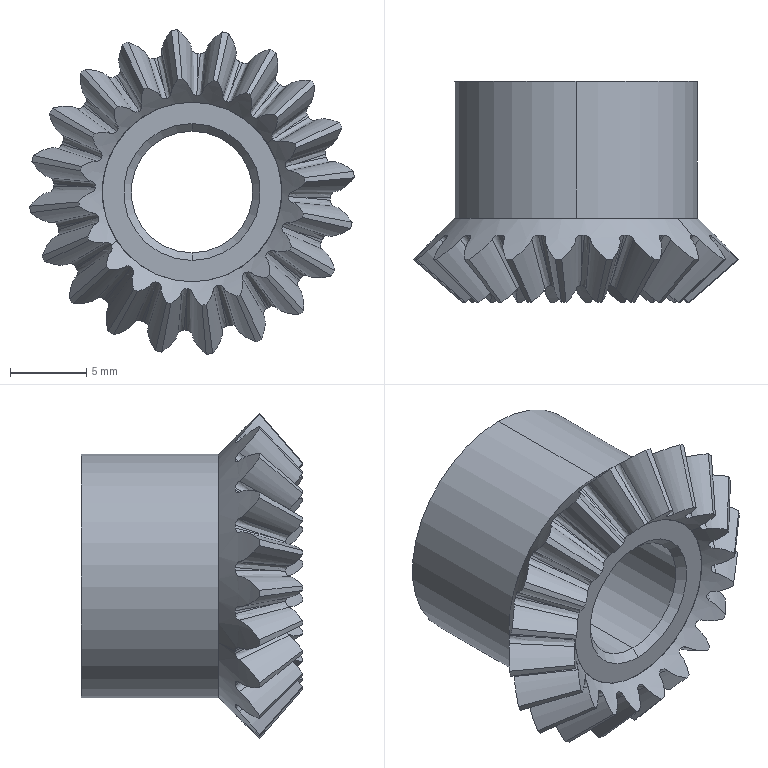Part | SolidWorks | features BaseBody 2 | 2 solids | 140 faces | box 21.332 x 14.53 x 21.332 mm | volume 2201 mm3 | spline 100 | cone 28 | cylinder 8 | plane 4 | commonest cylinder face diameters 11.8 x4 8 x2 16 x2